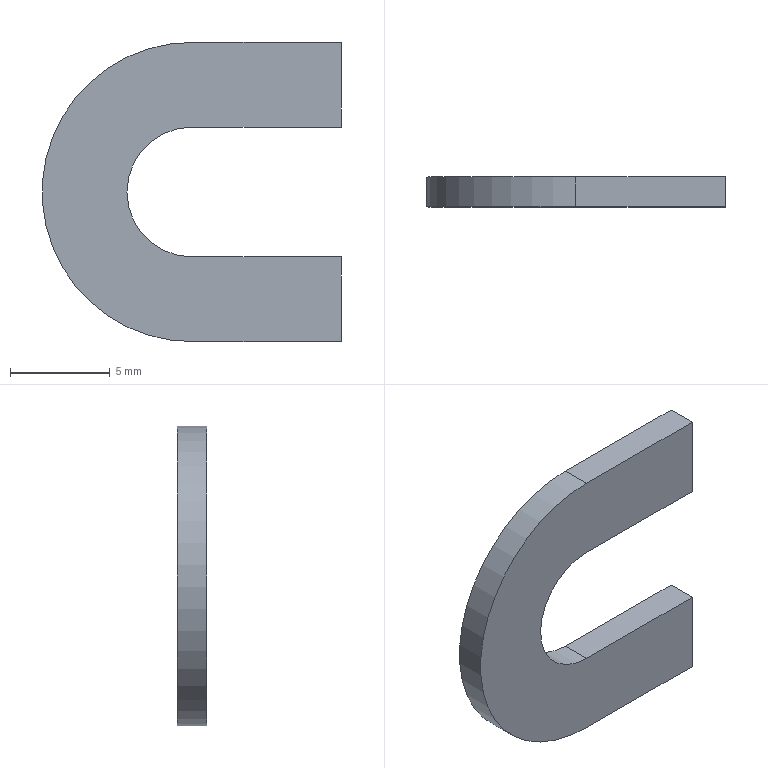Part | SolidWorks | features BaseBody 1 | 1 solid | 10 faces | box 15 x 1.5 x 15 mm | volume 203.274 mm3 | plane 8 | cylinder 2 | commonest cylinder face diameters 6.5 x1 15 x1
STEP:
#1=CARTESIAN_POINT('',(-28.901,46.92,48.25));
#2=VERTEX_POINT('',#1);
#3=CARTESIAN_POINT('',(-28.901,46.92,41.75));
#4=VERTEX_POINT('',#3);
#5=CARTESIAN_POINT('',(-28.901,46.92,45.));
#6=DIRECTION('',(0.,-1.,0.));
#7=DIRECTION('',(0.,0.,-1.));
#8=AXIS2_PLACEMENT_3D('',#5,#6,#7);
#9=CIRCLE('',#8,3.25);
#10=EDGE_CURVE('',#2,#4,#9,.T.);
#11=ORIENTED_EDGE('',*,*,#10,.F.);
#12=CARTESIAN_POINT('',(-21.401,46.92,48.25));
#13=VERTEX_POINT('',#12);
#14=CARTESIAN_POINT('',(-28.901,46.92,48.25));
#15=DIRECTION('',(-1.,0.,0.));
#16=VECTOR('',#15,1000.);
#17=LINE('',#14,#16);
#18=EDGE_CURVE('',#13,#2,#17,.T.);
#19=ORIENTED_EDGE('',*,*,#18,.F.);
#20=CARTESIAN_POINT('',(-21.401,46.92,52.5));
#21=VERTEX_POINT('',#20);
#22=CARTESIAN_POINT('',(-21.401,46.92,45.));
#23=DIRECTION('',(0.,0.,-1.));
#24=VECTOR('',#23,1000.);
#25=LINE('',#22,#24);
#26=EDGE_CURVE('',#21,#13,#25,.T.);
#27=ORIENTED_EDGE('',*,*,#26,.F.);
#28=CARTESIAN_POINT('',(-28.901,46.92,52.5));
#29=VERTEX_POINT('',#28);
#30=CARTESIAN_POINT('',(-28.901,46.92,52.5));
#31=DIRECTION('',(1.,0.,0.));
#32=VECTOR('',#31,1000.);
#33=LINE('',#30,#32);
#34=EDGE_CURVE('',#29,#21,#33,.T.);
#35=ORIENTED_EDGE('',*,*,#34,.F.);
#36=CARTESIAN_POINT('',(-28.901,46.92,37.5));
#37=VERTEX_POINT('',#36);
#38=CARTESIAN_POINT('',(-28.901,46.92,45.));
#39=DIRECTION('',(0.,1.,0.));
#40=DIRECTION('',(0.,0.,-1.));
#41=AXIS2_PLACEMENT_3D('',#38,#39,#40);
#42=CIRCLE('',#41,7.5);
#43=EDGE_CURVE('',#37,#29,#42,.T.);
#44=ORIENTED_EDGE('',*,*,#43,.F.);
#45=CARTESIAN_POINT('',(-21.401,46.92,37.5));
#46=VERTEX_POINT('',#45);
#47=CARTESIAN_POINT('',(-28.901,46.92,37.5));
#48=DIRECTION('',(-1.,0.,0.));
#49=VECTOR('',#48,1000.);
#50=LINE('',#47,#49);
#51=EDGE_CURVE('',#46,#37,#50,.T.);
#52=ORIENTED_EDGE('',*,*,#51,.F.);
#53=CARTESIAN_POINT('',(-21.401,46.92,41.75));
#54=VERTEX_POINT('',#53);
#55=CARTESIAN_POINT('',(-21.401,46.92,45.));
#56=DIRECTION('',(0.,0.,-1.));
#57=VECTOR('',#56,1000.);
#58=LINE('',#55,#57);
#59=EDGE_CURVE('',#54,#46,#58,.T.);
#60=ORIENTED_EDGE('',*,*,#59,.F.);
#61=CARTESIAN_POINT('',(-28.901,46.92,41.75));
#62=DIRECTION('',(1.,0.,0.));
#63=VECTOR('',#62,1000.);
#64=LINE('',#61,#63);
#65=EDGE_CURVE('',#4,#54,#64,.T.);
#66=ORIENTED_EDGE('',*,*,#65,.F.);
#67=EDGE_LOOP('',(#11,#19,#27,#35,#44,#52,#60,#66));
#68=FACE_OUTER_BOUND('',#67,.T.);
#69=CARTESIAN_POINT('',(-28.901,46.92,45.));
#70=DIRECTION('',(0.,1.,0.));
#71=DIRECTION('',(0.,0.,1.));
#72=AXIS2_PLACEMENT_3D('',#69,#70,#71);
#73=PLANE('',#72);
#74=ADVANCED_FACE('',(#68),#73,.F.);
#75=ORIENTED_EDGE('',*,*,#65,.T.);
#76=CARTESIAN_POINT('',(-21.401,48.42,41.75));
#77=VERTEX_POINT('',#76);
#78=CARTESIAN_POINT('',(-21.401,47.67,41.75));
#79=DIRECTION('',(0.,1.,0.));
#80=VECTOR('',#79,1000.);
#81=LINE('',#78,#80);
#82=EDGE_CURVE('',#54,#77,#81,.T.);
#83=ORIENTED_EDGE('',*,*,#82,.T.);
#84=CARTESIAN_POINT('',(-28.901,48.42,41.75));
#85=VERTEX_POINT('',#84);
#86=CARTESIAN_POINT('',(-25.151,48.42,41.75));
#87=DIRECTION('',(-1.,0.,0.));
#88=VECTOR('',#87,1000.);
#89=LINE('',#86,#88);
#90=EDGE_CURVE('',#77,#85,#89,.T.);
#91=ORIENTED_EDGE('',*,*,#90,.T.);
#92=CARTESIAN_POINT('',(-28.901,47.67,41.75));
#93=DIRECTION('',(0.,-1.,0.));
#94=VECTOR('',#93,1000.);
#95=LINE('',#92,#94);
#96=EDGE_CURVE('',#85,#4,#95,.T.);
#97=ORIENTED_EDGE('',*,*,#96,.T.);
#98=EDGE_LOOP('',(#75,#83,#91,#97));
#99=FACE_OUTER_BOUND('',#98,.T.);
#100=CARTESIAN_POINT('',(-25.151,47.67,41.75));
#101=DIRECTION('',(0.,0.,1.));
#102=DIRECTION('',(1.,0.,0.));
#103=AXIS2_PLACEMENT_3D('',#100,#101,#102);
#104=PLANE('',#103);
#105=ADVANCED_FACE('',(#99),#104,.T.);
#106=ORIENTED_EDGE('',*,*,#96,.F.);
#107=CARTESIAN_POINT('',(-28.901,48.42,48.25));
#108=VERTEX_POINT('',#107);
#109=CARTESIAN_POINT('',(-28.901,48.42,45.));
#110=DIRECTION('',(0.,-1.,0.));
#111=DIRECTION('',(0.,0.,-1.));
#112=AXIS2_PLACEMENT_3D('',#109,#110,#111);
#113=CIRCLE('',#112,3.25);
#114=EDGE_CURVE('',#108,#85,#113,.T.);
#115=ORIENTED_EDGE('',*,*,#114,.F.);
#116=CARTESIAN_POINT('',(-28.901,48.42,48.25));
#117=DIRECTION('',(0.,1.,0.));
#118=VECTOR('',#117,1000.);
#119=LINE('',#116,#118);
#120=EDGE_CURVE('',#2,#108,#119,.T.);
#121=ORIENTED_EDGE('',*,*,#120,.F.);
#122=ORIENTED_EDGE('',*,*,#10,.T.);
#123=EDGE_LOOP('',(#106,#115,#121,#122));
#124=FACE_OUTER_BOUND('',#123,.T.);
#125=CARTESIAN_POINT('',(-28.901,48.42,45.));
#126=DIRECTION('',(0.,-1.,0.));
#127=DIRECTION('',(0.,0.,-1.));
#128=AXIS2_PLACEMENT_3D('',#125,#126,#127);
#129=CYLINDRICAL_SURFACE('',#128,3.25);
#130=ADVANCED_FACE('',(#124),#129,.F.);
#131=ORIENTED_EDGE('',*,*,#18,.T.);
#132=ORIENTED_EDGE('',*,*,#120,.T.);
#133=CARTESIAN_POINT('',(-21.401,48.42,48.25));
#134=VERTEX_POINT('',#133);
#135=CARTESIAN_POINT('',(-25.151,48.42,48.25));
#136=DIRECTION('',(-1.,0.,0.));
#137=VECTOR('',#136,1000.);
#138=LINE('',#135,#137);
#139=EDGE_CURVE('',#134,#108,#138,.T.);
#140=ORIENTED_EDGE('',*,*,#139,.F.);
#141=CARTESIAN_POINT('',(-21.401,47.67,48.25));
#142=DIRECTION('',(0.,1.,0.));
#143=VECTOR('',#142,1000.);
#144=LINE('',#141,#143);
#145=EDGE_CURVE('',#13,#134,#144,.T.);
#146=ORIENTED_EDGE('',*,*,#145,.F.);
#147=EDGE_LOOP('',(#131,#132,#140,#146));
#148=FACE_OUTER_BOUND('',#147,.T.);
#149=CARTESIAN_POINT('',(-25.151,47.67,48.25));
#150=DIRECTION('',(0.,0.,1.));
#151=DIRECTION('',(1.,0.,0.));
#152=AXIS2_PLACEMENT_3D('',#149,#150,#151);
#153=PLANE('',#152);
#154=ADVANCED_FACE('',(#148),#153,.F.);
#155=ORIENTED_EDGE('',*,*,#26,.T.);
#156=ORIENTED_EDGE('',*,*,#145,.T.);
#157=CARTESIAN_POINT('',(-21.401,48.42,52.5));
#158=VERTEX_POINT('',#157);
#159=CARTESIAN_POINT('',(-21.401,48.42,50.375));
#160=DIRECTION('',(0.,0.,1.));
#161=VECTOR('',#160,1000.);
#162=LINE('',#159,#161);
#163=EDGE_CURVE('',#134,#158,#162,.T.);
#164=ORIENTED_EDGE('',*,*,#163,.T.);
#165=CARTESIAN_POINT('',(-21.401,47.67,52.5));
#166=DIRECTION('',(0.,-1.,0.));
#167=VECTOR('',#166,1000.);
#168=LINE('',#165,#167);
#169=EDGE_CURVE('',#158,#21,#168,.T.);
#170=ORIENTED_EDGE('',*,*,#169,.T.);
#171=EDGE_LOOP('',(#155,#156,#164,#170));
#172=FACE_OUTER_BOUND('',#171,.T.);
#173=CARTESIAN_POINT('',(-21.401,47.67,50.375));
#174=DIRECTION('',(1.,0.,0.));
#175=DIRECTION('',(0.,0.,-1.));
#176=AXIS2_PLACEMENT_3D('',#173,#174,#175);
#177=PLANE('',#176);
#178=ADVANCED_FACE('',(#172),#177,.T.);
#179=ORIENTED_EDGE('',*,*,#34,.T.);
#180=ORIENTED_EDGE('',*,*,#169,.F.);
#181=CARTESIAN_POINT('',(-28.901,48.42,52.5));
#182=VERTEX_POINT('',#181);
#183=CARTESIAN_POINT('',(-25.151,48.42,52.5));
#184=DIRECTION('',(-1.,0.,0.));
#185=VECTOR('',#184,1000.);
#186=LINE('',#183,#185);
#187=EDGE_CURVE('',#158,#182,#186,.T.);
#188=ORIENTED_EDGE('',*,*,#187,.T.);
#189=CARTESIAN_POINT('',(-28.901,47.67,52.5));
#190=DIRECTION('',(0.,-1.,0.));
#191=VECTOR('',#190,1000.);
#192=LINE('',#189,#191);
#193=EDGE_CURVE('',#182,#29,#192,.T.);
#194=ORIENTED_EDGE('',*,*,#193,.T.);
#195=EDGE_LOOP('',(#179,#180,#188,#194));
#196=FACE_OUTER_BOUND('',#195,.T.);
#197=CARTESIAN_POINT('',(-25.151,47.67,52.5));
#198=DIRECTION('',(0.,0.,1.));
#199=DIRECTION('',(1.,0.,0.));
#200=AXIS2_PLACEMENT_3D('',#197,#198,#199);
#201=PLANE('',#200);
#202=ADVANCED_FACE('',(#196),#201,.T.);
#203=CARTESIAN_POINT('',(-28.901,48.42,37.5));
#204=VERTEX_POINT('',#203);
#205=CARTESIAN_POINT('',(-28.901,47.67,37.5));
#206=DIRECTION('',(0.,-1.,0.));
#207=VECTOR('',#206,1000.);
#208=LINE('',#205,#207);
#209=EDGE_CURVE('',#204,#37,#208,.T.);
#210=ORIENTED_EDGE('',*,*,#209,.T.);
#211=ORIENTED_EDGE('',*,*,#43,.T.);
#212=ORIENTED_EDGE('',*,*,#193,.F.);
#213=CARTESIAN_POINT('',(-28.901,48.42,45.));
#214=DIRECTION('',(0.,-1.,0.));
#215=DIRECTION('',(0.,0.,-1.));
#216=AXIS2_PLACEMENT_3D('',#213,#214,#215);
#217=CIRCLE('',#216,7.5);
#218=EDGE_CURVE('',#182,#204,#217,.T.);
#219=ORIENTED_EDGE('',*,*,#218,.T.);
#220=EDGE_LOOP('',(#210,#211,#212,#219));
#221=FACE_OUTER_BOUND('',#220,.T.);
#222=CARTESIAN_POINT('',(-28.901,48.42,45.));
#223=DIRECTION('',(0.,-1.,0.));
#224=DIRECTION('',(0.,0.,-1.));
#225=AXIS2_PLACEMENT_3D('',#222,#223,#224);
#226=CYLINDRICAL_SURFACE('',#225,7.5);
#227=ADVANCED_FACE('',(#221),#226,.T.);
#228=ORIENTED_EDGE('',*,*,#51,.T.);
#229=ORIENTED_EDGE('',*,*,#209,.F.);
#230=CARTESIAN_POINT('',(-21.401,48.42,37.5));
#231=VERTEX_POINT('',#230);
#232=CARTESIAN_POINT('',(-25.151,48.42,37.5));
#233=DIRECTION('',(-1.,0.,0.));
#234=VECTOR('',#233,1000.);
#235=LINE('',#232,#234);
#236=EDGE_CURVE('',#231,#204,#235,.T.);
#237=ORIENTED_EDGE('',*,*,#236,.F.);
#238=CARTESIAN_POINT('',(-21.401,47.67,37.5));
#239=DIRECTION('',(0.,1.,0.));
#240=VECTOR('',#239,1000.);
#241=LINE('',#238,#240);
#242=EDGE_CURVE('',#46,#231,#241,.T.);
#243=ORIENTED_EDGE('',*,*,#242,.F.);
#244=EDGE_LOOP('',(#228,#229,#237,#243));
#245=FACE_OUTER_BOUND('',#244,.T.);
#246=CARTESIAN_POINT('',(-25.151,47.67,37.5));
#247=DIRECTION('',(0.,0.,1.));
#248=DIRECTION('',(1.,0.,0.));
#249=AXIS2_PLACEMENT_3D('',#246,#247,#248);
#250=PLANE('',#249);
#251=ADVANCED_FACE('',(#245),#250,.F.);
#252=ORIENTED_EDGE('',*,*,#59,.T.);
#253=ORIENTED_EDGE('',*,*,#242,.T.);
#254=CARTESIAN_POINT('',(-21.401,48.42,39.625));
#255=DIRECTION('',(0.,0.,1.));
#256=VECTOR('',#255,1000.);
#257=LINE('',#254,#256);
#258=EDGE_CURVE('',#231,#77,#257,.T.);
#259=ORIENTED_EDGE('',*,*,#258,.T.);
#260=ORIENTED_EDGE('',*,*,#82,.F.);
#261=EDGE_LOOP('',(#252,#253,#259,#260));
#262=FACE_OUTER_BOUND('',#261,.T.);
#263=CARTESIAN_POINT('',(-21.401,47.67,39.625));
#264=DIRECTION('',(1.,0.,0.));
#265=DIRECTION('',(0.,0.,-1.));
#266=AXIS2_PLACEMENT_3D('',#263,#264,#265);
#267=PLANE('',#266);
#268=ADVANCED_FACE('',(#262),#267,.T.);
#269=ORIENTED_EDGE('',*,*,#114,.T.);
#270=ORIENTED_EDGE('',*,*,#90,.F.);
#271=ORIENTED_EDGE('',*,*,#258,.F.);
#272=ORIENTED_EDGE('',*,*,#236,.T.);
#273=ORIENTED_EDGE('',*,*,#218,.F.);
#274=ORIENTED_EDGE('',*,*,#187,.F.);
#275=ORIENTED_EDGE('',*,*,#163,.F.);
#276=ORIENTED_EDGE('',*,*,#139,.T.);
#277=EDGE_LOOP('',(#269,#270,#271,#272,#273,#274,#275,#276));
#278=FACE_OUTER_BOUND('',#277,.T.);
#279=CARTESIAN_POINT('',(-28.901,48.42,45.));
#280=DIRECTION('',(0.,1.,0.));
#281=DIRECTION('',(0.,0.,1.));
#282=AXIS2_PLACEMENT_3D('',#279,#280,#281);
#283=PLANE('',#282);
#284=ADVANCED_FACE('',(#278),#283,.T.);
#285=CLOSED_SHELL('',(#74,#105,#130,#154,#178,#202,#227,#251,#268,#284));
#286=MANIFOLD_SOLID_BREP('',#285);
#287=CARTESIAN_POINT('',(0.,0.,0.));
#288=DIRECTION('',(0.,0.,1.));
#289=DIRECTION('',(1.,0.,0.));
#290=AXIS2_PLACEMENT_3D('',#287,#288,#289);
#291=(LENGTH_UNIT()NAMED_UNIT(*)SI_UNIT(.MILLI.,.METRE.));
#292=UNCERTAINTY_MEASURE_WITH_UNIT(LENGTH_MEASURE(0.00001),#291,'','');
#293=(NAMED_UNIT(*)PLANE_ANGLE_UNIT()SI_UNIT($,.RADIAN.));
#294=(NAMED_UNIT(*)SI_UNIT($,.STERADIAN.)SOLID_ANGLE_UNIT());
#295=(GEOMETRIC_REPRESENTATION_CONTEXT(3)GLOBAL_UNCERTAINTY_ASSIGNED_CONTEXT((#292))GLOBAL_UNIT_ASSIGNED_CONTEXT((#291,#293,#294))REPRESENTATION_CONTEXT('',''));
#296=ADVANCED_BREP_SHAPE_REPRESENTATION('',(#286,#290),#295);